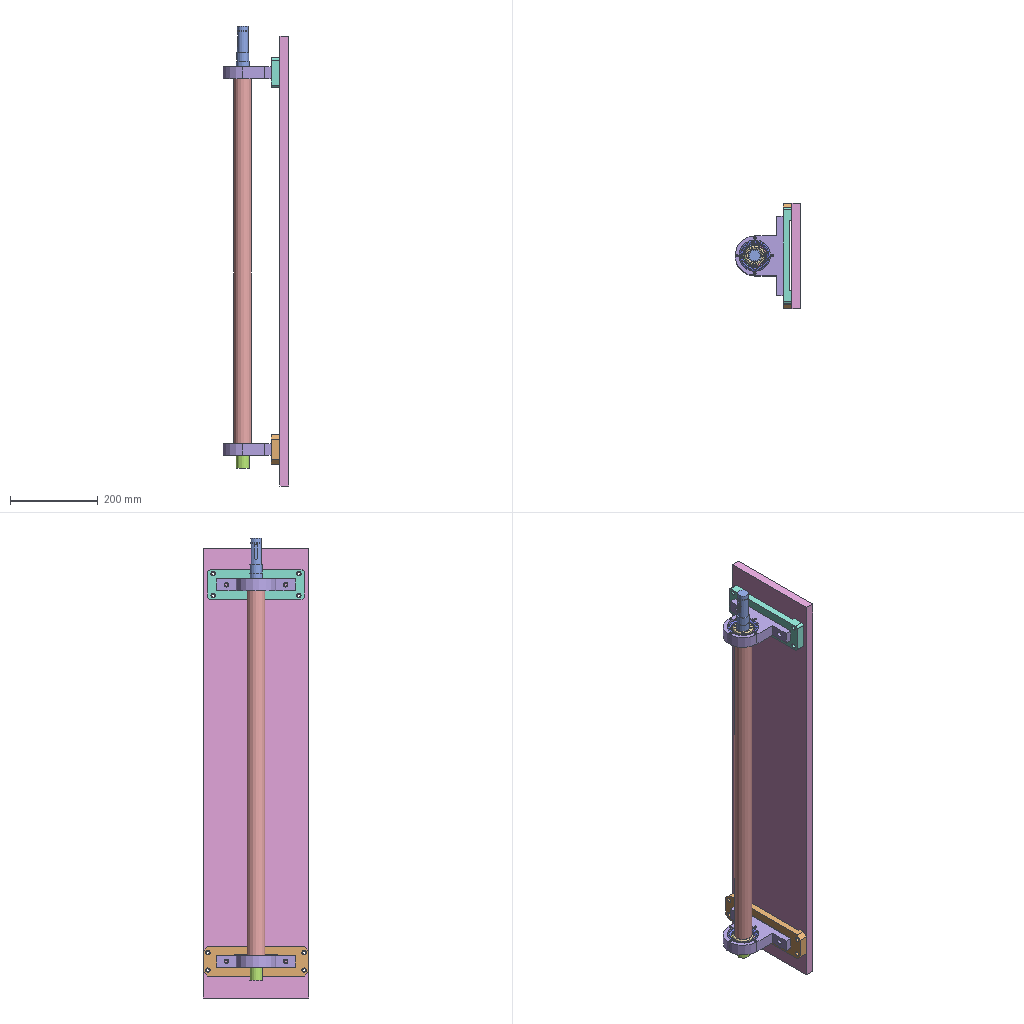Assembly | NX | 7 different items | 9 placed | box 149 x 240 x 1050 mm
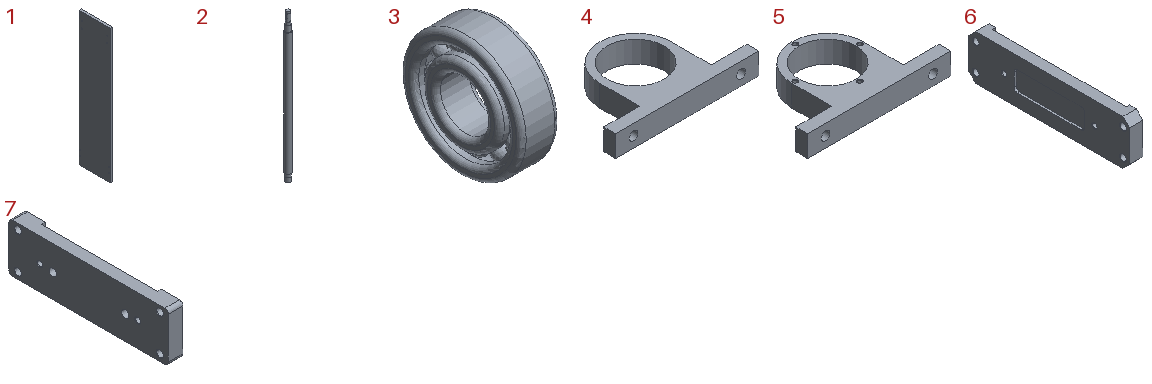Parts list (item | quantity | size | volume | features):
1 | x1 | 20 x 240 x 1027 mm | 4923724 mm3 | features SIMPLE HOLE 8, SYMBOLIC_THREAD 8, LINKED_CURVE 4, DATUM_CSYS 3, SKETCH 2, EXTRUDE 1, HOLE PACKAGE 1, LINKED_FACE 1
2 | x1 | - | 1157120 mm3 | features EXTRUDE 8, DATUM_CSYS 5, SKETCH 4, EXTRACT_DATUM_AXIS 2, CPROJ 1, DATUM_PLANE 1, EXTRACT_DATUM_PLANE 1, LINKED_POINT 1
3 | x2 | 23 x 72 x 72 mm | 56238 mm3 | features EXTRACT_BODY 12, BLEND 3, DATUM_CSYS 3, SKETCH 2, Container 1, EXTRUDE 1, Geometry Instance 1, Pattern Geometry 1, SHELL 1, SPHERE 1, SUBTRACT 1, SWP104 1
4 | x1 | 180 x 110 x 27 mm | 166653 mm3 | features DATUM_CSYS 5, SKETCH 4, EXTRUDE 3
5 | x2 | 180 x 110 x 27 mm | 165663 mm3 | features DATUM_CSYS 9, SKETCH 8, EXTRACT_FACE 4, HOLE PACKAGE 4, SIMPLE HOLE 4, SYMBOLIC_THREAD 4, EXTRUDE 3, Instance Feature 3, Pattern Feature 1
6 | x1 | 20 x 240 x 67 mm | 234977 mm3 | features DATUM_CSYS 6, SIMPLE HOLE 6, SKETCH 5, EXTRUDE 3, HOLE PACKAGE 2, LINKED_CURVE 2, SYMBOLIC_THREAD 2, BLEND 1, CHAMFER 1, LINKED_FACE 1
7 | x1 | 20 x 220 x 67 mm | 225949 mm3 | features SIMPLE HOLE 8, DATUM_CSYS 7, SKETCH 6, EXTRUDE 3, HOLE PACKAGE 3, BLEND 2, SYMBOLIC_THREAD 2, LINKED_CURVE 1, LINKED_FACE 1